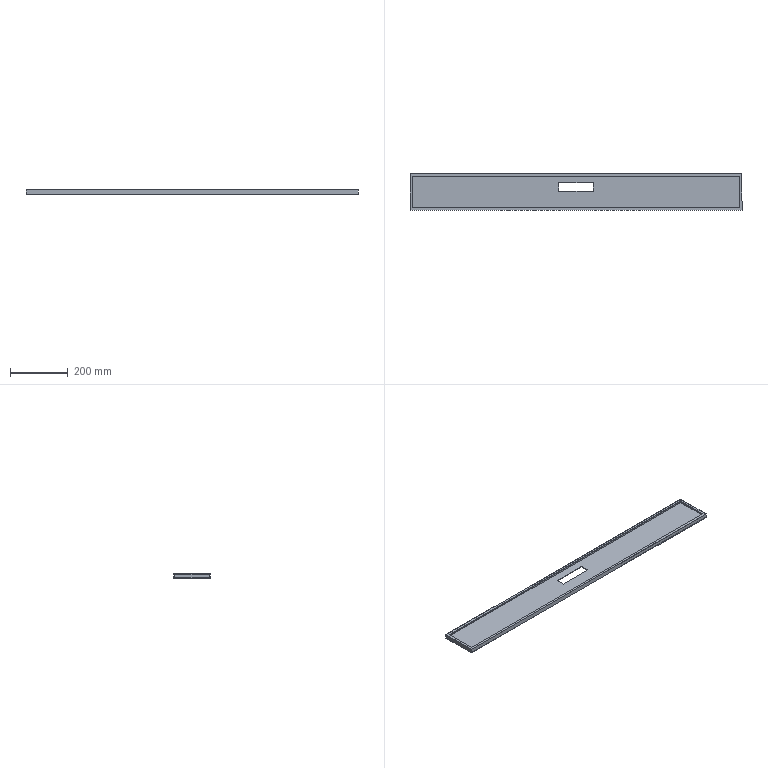Part | SolidWorks | features ICE 2, Extrusion 1, Shell 1 | 1 solid | 20 faces | box 1148 x 125 x 15 mm | volume 375860 mm3 | plane 20
STEP:
#1=CARTESIAN_POINT('',(0.,125.,15.));
#2=VERTEX_POINT('',#1);
#3=CARTESIAN_POINT('',(0.,0.,15.));
#4=VERTEX_POINT('',#3);
#5=CARTESIAN_POINT('',(0.,0.,15.));
#6=DIRECTION('',(0.,-1.,0.));
#7=VECTOR('',#6,1000.);
#8=LINE('',#5,#7);
#9=EDGE_CURVE('',#2,#4,#8,.T.);
#10=ORIENTED_EDGE('',*,*,#9,.T.);
#11=CARTESIAN_POINT('',(1148.,0.,15.));
#12=VERTEX_POINT('',#11);
#13=CARTESIAN_POINT('',(0.,0.,15.));
#14=DIRECTION('',(1.,0.,0.));
#15=VECTOR('',#14,1000.);
#16=LINE('',#13,#15);
#17=EDGE_CURVE('',#4,#12,#16,.T.);
#18=ORIENTED_EDGE('',*,*,#17,.T.);
#19=CARTESIAN_POINT('',(1148.,125.,15.));
#20=VERTEX_POINT('',#19);
#21=CARTESIAN_POINT('',(1148.,0.,15.));
#22=DIRECTION('',(0.,1.,0.));
#23=VECTOR('',#22,1000.);
#24=LINE('',#21,#23);
#25=EDGE_CURVE('',#12,#20,#24,.T.);
#26=ORIENTED_EDGE('',*,*,#25,.T.);
#27=CARTESIAN_POINT('',(0.,125.,15.));
#28=DIRECTION('',(-1.,0.,0.));
#29=VECTOR('',#28,1000.);
#30=LINE('',#27,#29);
#31=EDGE_CURVE('',#20,#2,#30,.T.);
#32=ORIENTED_EDGE('',*,*,#31,.T.);
#33=EDGE_LOOP('',(#10,#18,#26,#32));
#34=FACE_OUTER_BOUND('',#33,.T.);
#35=CARTESIAN_POINT('',(1140.,117.,15.));
#36=VERTEX_POINT('',#35);
#37=CARTESIAN_POINT('',(8.,117.,15.));
#38=VERTEX_POINT('',#37);
#39=CARTESIAN_POINT('',(8.,117.,15.));
#40=DIRECTION('',(-1.,0.,0.));
#41=VECTOR('',#40,1000.);
#42=LINE('',#39,#41);
#43=EDGE_CURVE('',#36,#38,#42,.T.);
#44=ORIENTED_EDGE('',*,*,#43,.F.);
#45=CARTESIAN_POINT('',(1140.,8.,15.));
#46=VERTEX_POINT('',#45);
#47=CARTESIAN_POINT('',(1140.,117.,15.));
#48=DIRECTION('',(0.,1.,0.));
#49=VECTOR('',#48,1000.);
#50=LINE('',#47,#49);
#51=EDGE_CURVE('',#46,#36,#50,.T.);
#52=ORIENTED_EDGE('',*,*,#51,.F.);
#53=CARTESIAN_POINT('',(8.,8.,15.));
#54=VERTEX_POINT('',#53);
#55=CARTESIAN_POINT('',(8.,8.,15.));
#56=DIRECTION('',(1.,0.,0.));
#57=VECTOR('',#56,1000.);
#58=LINE('',#55,#57);
#59=EDGE_CURVE('',#54,#46,#58,.T.);
#60=ORIENTED_EDGE('',*,*,#59,.F.);
#61=CARTESIAN_POINT('',(8.,117.,15.));
#62=DIRECTION('',(0.,-1.,0.));
#63=VECTOR('',#62,1000.);
#64=LINE('',#61,#63);
#65=EDGE_CURVE('',#38,#54,#64,.T.);
#66=ORIENTED_EDGE('',*,*,#65,.F.);
#67=EDGE_LOOP('',(#44,#52,#60,#66));
#68=FACE_BOUND('',#67,.T.);
#69=CARTESIAN_POINT('',(0.,125.,15.));
#70=DIRECTION('',(0.,0.,-1.));
#71=DIRECTION('',(-1.,0.,0.));
#72=AXIS2_PLACEMENT_3D('',#69,#70,#71);
#73=PLANE('',#72);
#74=ADVANCED_FACE('',(#34,#68),#73,.F.);
#75=CARTESIAN_POINT('',(0.,125.,0.));
#76=VERTEX_POINT('',#75);
#77=CARTESIAN_POINT('',(0.,125.,15.));
#78=DIRECTION('',(0.,0.,-1.));
#79=VECTOR('',#78,1000.);
#80=LINE('',#77,#79);
#81=EDGE_CURVE('',#2,#76,#80,.T.);
#82=ORIENTED_EDGE('',*,*,#81,.T.);
#83=CARTESIAN_POINT('',(0.,0.,0.));
#84=VERTEX_POINT('',#83);
#85=CARTESIAN_POINT('',(0.,0.,0.));
#86=DIRECTION('',(0.,-1.,0.));
#87=VECTOR('',#86,1000.);
#88=LINE('',#85,#87);
#89=EDGE_CURVE('',#76,#84,#88,.T.);
#90=ORIENTED_EDGE('',*,*,#89,.T.);
#91=CARTESIAN_POINT('',(0.,0.,15.));
#92=DIRECTION('',(0.,0.,-1.));
#93=VECTOR('',#92,1000.);
#94=LINE('',#91,#93);
#95=EDGE_CURVE('',#4,#84,#94,.T.);
#96=ORIENTED_EDGE('',*,*,#95,.F.);
#97=ORIENTED_EDGE('',*,*,#9,.F.);
#98=EDGE_LOOP('',(#82,#90,#96,#97));
#99=FACE_OUTER_BOUND('',#98,.T.);
#100=CARTESIAN_POINT('',(0.,0.,15.));
#101=DIRECTION('',(1.,0.,0.));
#102=DIRECTION('',(0.,0.,-1.));
#103=AXIS2_PLACEMENT_3D('',#100,#101,#102);
#104=PLANE('',#103);
#105=ADVANCED_FACE('',(#99),#104,.F.);
#106=ORIENTED_EDGE('',*,*,#95,.T.);
#107=CARTESIAN_POINT('',(1148.,0.,0.));
#108=VERTEX_POINT('',#107);
#109=CARTESIAN_POINT('',(0.,0.,0.));
#110=DIRECTION('',(1.,0.,0.));
#111=VECTOR('',#110,1000.);
#112=LINE('',#109,#111);
#113=EDGE_CURVE('',#84,#108,#112,.T.);
#114=ORIENTED_EDGE('',*,*,#113,.T.);
#115=CARTESIAN_POINT('',(1148.,0.,15.));
#116=DIRECTION('',(0.,0.,-1.));
#117=VECTOR('',#116,1000.);
#118=LINE('',#115,#117);
#119=EDGE_CURVE('',#12,#108,#118,.T.);
#120=ORIENTED_EDGE('',*,*,#119,.F.);
#121=ORIENTED_EDGE('',*,*,#17,.F.);
#122=EDGE_LOOP('',(#106,#114,#120,#121));
#123=FACE_OUTER_BOUND('',#122,.T.);
#124=CARTESIAN_POINT('',(0.,0.,15.));
#125=DIRECTION('',(0.,1.,0.));
#126=DIRECTION('',(0.,0.,1.));
#127=AXIS2_PLACEMENT_3D('',#124,#125,#126);
#128=PLANE('',#127);
#129=ADVANCED_FACE('',(#123),#128,.F.);
#130=ORIENTED_EDGE('',*,*,#119,.T.);
#131=CARTESIAN_POINT('',(1148.,125.,0.));
#132=VERTEX_POINT('',#131);
#133=CARTESIAN_POINT('',(1148.,0.,0.));
#134=DIRECTION('',(0.,1.,0.));
#135=VECTOR('',#134,1000.);
#136=LINE('',#133,#135);
#137=EDGE_CURVE('',#108,#132,#136,.T.);
#138=ORIENTED_EDGE('',*,*,#137,.T.);
#139=CARTESIAN_POINT('',(1148.,125.,15.));
#140=DIRECTION('',(0.,0.,-1.));
#141=VECTOR('',#140,1000.);
#142=LINE('',#139,#141);
#143=EDGE_CURVE('',#20,#132,#142,.T.);
#144=ORIENTED_EDGE('',*,*,#143,.F.);
#145=ORIENTED_EDGE('',*,*,#25,.F.);
#146=EDGE_LOOP('',(#130,#138,#144,#145));
#147=FACE_OUTER_BOUND('',#146,.T.);
#148=CARTESIAN_POINT('',(1148.,0.,15.));
#149=DIRECTION('',(-1.,0.,0.));
#150=DIRECTION('',(0.,-1.,0.));
#151=AXIS2_PLACEMENT_3D('',#148,#149,#150);
#152=PLANE('',#151);
#153=ADVANCED_FACE('',(#147),#152,.F.);
#154=ORIENTED_EDGE('',*,*,#143,.T.);
#155=CARTESIAN_POINT('',(0.,125.,0.));
#156=DIRECTION('',(-1.,0.,0.));
#157=VECTOR('',#156,1000.);
#158=LINE('',#155,#157);
#159=EDGE_CURVE('',#132,#76,#158,.T.);
#160=ORIENTED_EDGE('',*,*,#159,.T.);
#161=ORIENTED_EDGE('',*,*,#81,.F.);
#162=ORIENTED_EDGE('',*,*,#31,.F.);
#163=EDGE_LOOP('',(#154,#160,#161,#162));
#164=FACE_OUTER_BOUND('',#163,.T.);
#165=CARTESIAN_POINT('',(0.,125.,15.));
#166=DIRECTION('',(0.,-1.,0.));
#167=DIRECTION('',(0.,0.,-1.));
#168=AXIS2_PLACEMENT_3D('',#165,#166,#167);
#169=PLANE('',#168);
#170=ADVANCED_FACE('',(#164),#169,.F.);
#171=CARTESIAN_POINT('',(634.,95.,0.));
#172=VERTEX_POINT('',#171);
#173=CARTESIAN_POINT('',(634.,65.,0.));
#174=VERTEX_POINT('',#173);
#175=CARTESIAN_POINT('',(634.,95.,0.));
#176=DIRECTION('',(0.,-1.,0.));
#177=VECTOR('',#176,1000.);
#178=LINE('',#175,#177);
#179=EDGE_CURVE('',#172,#174,#178,.T.);
#180=ORIENTED_EDGE('',*,*,#179,.F.);
#181=CARTESIAN_POINT('',(514.,95.,0.));
#182=VERTEX_POINT('',#181);
#183=CARTESIAN_POINT('',(634.,95.,0.));
#184=DIRECTION('',(1.,0.,0.));
#185=VECTOR('',#184,1000.);
#186=LINE('',#183,#185);
#187=EDGE_CURVE('',#182,#172,#186,.T.);
#188=ORIENTED_EDGE('',*,*,#187,.F.);
#189=CARTESIAN_POINT('',(514.,65.,0.));
#190=VERTEX_POINT('',#189);
#191=CARTESIAN_POINT('',(514.,95.,0.));
#192=DIRECTION('',(0.,1.,0.));
#193=VECTOR('',#192,1000.);
#194=LINE('',#191,#193);
#195=EDGE_CURVE('',#190,#182,#194,.T.);
#196=ORIENTED_EDGE('',*,*,#195,.F.);
#197=CARTESIAN_POINT('',(634.,65.,0.));
#198=DIRECTION('',(-1.,0.,0.));
#199=VECTOR('',#198,1000.);
#200=LINE('',#197,#199);
#201=EDGE_CURVE('',#174,#190,#200,.T.);
#202=ORIENTED_EDGE('',*,*,#201,.F.);
#203=EDGE_LOOP('',(#180,#188,#196,#202));
#204=FACE_BOUND('',#203,.T.);
#205=ORIENTED_EDGE('',*,*,#89,.F.);
#206=ORIENTED_EDGE('',*,*,#159,.F.);
#207=ORIENTED_EDGE('',*,*,#137,.F.);
#208=ORIENTED_EDGE('',*,*,#113,.F.);
#209=EDGE_LOOP('',(#205,#206,#207,#208));
#210=FACE_OUTER_BOUND('',#209,.T.);
#211=CARTESIAN_POINT('',(0.,125.,0.));
#212=DIRECTION('',(0.,0.,-1.));
#213=DIRECTION('',(-1.,0.,0.));
#214=AXIS2_PLACEMENT_3D('',#211,#212,#213);
#215=PLANE('',#214);
#216=ADVANCED_FACE('',(#204,#210),#215,.T.);
#217=CARTESIAN_POINT('',(2.,123.,13.));
#218=VERTEX_POINT('',#217);
#219=CARTESIAN_POINT('',(2.,2.,13.));
#220=VERTEX_POINT('',#219);
#221=CARTESIAN_POINT('',(2.,0.,13.));
#222=DIRECTION('',(0.,-1.,0.));
#223=VECTOR('',#222,1000.);
#224=LINE('',#221,#223);
#225=EDGE_CURVE('',#218,#220,#224,.T.);
#226=ORIENTED_EDGE('',*,*,#225,.F.);
#227=CARTESIAN_POINT('',(1146.,123.,13.));
#228=VERTEX_POINT('',#227);
#229=CARTESIAN_POINT('',(0.,123.,13.));
#230=DIRECTION('',(-1.,0.,0.));
#231=VECTOR('',#230,1000.);
#232=LINE('',#229,#231);
#233=EDGE_CURVE('',#228,#218,#232,.T.);
#234=ORIENTED_EDGE('',*,*,#233,.F.);
#235=CARTESIAN_POINT('',(1146.,2.,13.));
#236=VERTEX_POINT('',#235);
#237=CARTESIAN_POINT('',(1146.,0.,13.));
#238=DIRECTION('',(0.,1.,0.));
#239=VECTOR('',#238,1000.);
#240=LINE('',#237,#239);
#241=EDGE_CURVE('',#236,#228,#240,.T.);
#242=ORIENTED_EDGE('',*,*,#241,.F.);
#243=CARTESIAN_POINT('',(0.,2.,13.));
#244=DIRECTION('',(1.,0.,0.));
#245=VECTOR('',#244,1000.);
#246=LINE('',#243,#245);
#247=EDGE_CURVE('',#220,#236,#246,.T.);
#248=ORIENTED_EDGE('',*,*,#247,.F.);
#249=EDGE_LOOP('',(#226,#234,#242,#248));
#250=FACE_OUTER_BOUND('',#249,.T.);
#251=CARTESIAN_POINT('',(1140.,8.,13.));
#252=VERTEX_POINT('',#251);
#253=CARTESIAN_POINT('',(1140.,117.,13.));
#254=VERTEX_POINT('',#253);
#255=CARTESIAN_POINT('',(1140.,117.,13.));
#256=DIRECTION('',(0.,1.,0.));
#257=VECTOR('',#256,1000.);
#258=LINE('',#255,#257);
#259=EDGE_CURVE('',#252,#254,#258,.T.);
#260=ORIENTED_EDGE('',*,*,#259,.T.);
#261=CARTESIAN_POINT('',(8.,117.,13.));
#262=VERTEX_POINT('',#261);
#263=CARTESIAN_POINT('',(8.,117.,13.));
#264=DIRECTION('',(-1.,0.,0.));
#265=VECTOR('',#264,1000.);
#266=LINE('',#263,#265);
#267=EDGE_CURVE('',#254,#262,#266,.T.);
#268=ORIENTED_EDGE('',*,*,#267,.T.);
#269=CARTESIAN_POINT('',(8.,8.,13.));
#270=VERTEX_POINT('',#269);
#271=CARTESIAN_POINT('',(8.,117.,13.));
#272=DIRECTION('',(0.,-1.,0.));
#273=VECTOR('',#272,1000.);
#274=LINE('',#271,#273);
#275=EDGE_CURVE('',#262,#270,#274,.T.);
#276=ORIENTED_EDGE('',*,*,#275,.T.);
#277=CARTESIAN_POINT('',(8.,8.,13.));
#278=DIRECTION('',(1.,0.,0.));
#279=VECTOR('',#278,1000.);
#280=LINE('',#277,#279);
#281=EDGE_CURVE('',#270,#252,#280,.T.);
#282=ORIENTED_EDGE('',*,*,#281,.T.);
#283=EDGE_LOOP('',(#260,#268,#276,#282));
#284=FACE_BOUND('',#283,.T.);
#285=CARTESIAN_POINT('',(0.,0.,13.));
#286=DIRECTION('',(0.,0.,1.));
#287=DIRECTION('',(1.,0.,0.));
#288=AXIS2_PLACEMENT_3D('',#285,#286,#287);
#289=PLANE('',#288);
#290=ADVANCED_FACE('',(#250,#284),#289,.F.);
#291=ORIENTED_EDGE('',*,*,#43,.T.);
#292=CARTESIAN_POINT('',(8.,117.,13.));
#293=DIRECTION('',(0.,0.,1.));
#294=VECTOR('',#293,1000.);
#295=LINE('',#292,#294);
#296=EDGE_CURVE('',#262,#38,#295,.T.);
#297=ORIENTED_EDGE('',*,*,#296,.F.);
#298=ORIENTED_EDGE('',*,*,#267,.F.);
#299=CARTESIAN_POINT('',(1140.,117.,13.));
#300=DIRECTION('',(0.,0.,1.));
#301=VECTOR('',#300,1000.);
#302=LINE('',#299,#301);
#303=EDGE_CURVE('',#254,#36,#302,.T.);
#304=ORIENTED_EDGE('',*,*,#303,.T.);
#305=EDGE_LOOP('',(#291,#297,#298,#304));
#306=FACE_OUTER_BOUND('',#305,.T.);
#307=CARTESIAN_POINT('',(8.,117.,13.));
#308=DIRECTION('',(0.,1.,0.));
#309=DIRECTION('',(0.,0.,1.));
#310=AXIS2_PLACEMENT_3D('',#307,#308,#309);
#311=PLANE('',#310);
#312=ADVANCED_FACE('',(#306),#311,.F.);
#313=ORIENTED_EDGE('',*,*,#51,.T.);
#314=ORIENTED_EDGE('',*,*,#303,.F.);
#315=ORIENTED_EDGE('',*,*,#259,.F.);
#316=CARTESIAN_POINT('',(1140.,8.,13.));
#317=DIRECTION('',(0.,0.,1.));
#318=VECTOR('',#317,1000.);
#319=LINE('',#316,#318);
#320=EDGE_CURVE('',#252,#46,#319,.T.);
#321=ORIENTED_EDGE('',*,*,#320,.T.);
#322=EDGE_LOOP('',(#313,#314,#315,#321));
#323=FACE_OUTER_BOUND('',#322,.T.);
#324=CARTESIAN_POINT('',(1140.,117.,13.));
#325=DIRECTION('',(1.,0.,0.));
#326=DIRECTION('',(0.,0.,-1.));
#327=AXIS2_PLACEMENT_3D('',#324,#325,#326);
#328=PLANE('',#327);
#329=ADVANCED_FACE('',(#323),#328,.F.);
#330=ORIENTED_EDGE('',*,*,#59,.T.);
#331=ORIENTED_EDGE('',*,*,#320,.F.);
#332=ORIENTED_EDGE('',*,*,#281,.F.);
#333=CARTESIAN_POINT('',(8.,8.,13.));
#334=DIRECTION('',(0.,0.,1.));
#335=VECTOR('',#334,1000.);
#336=LINE('',#333,#335);
#337=EDGE_CURVE('',#270,#54,#336,.T.);
#338=ORIENTED_EDGE('',*,*,#337,.T.);
#339=EDGE_LOOP('',(#330,#331,#332,#338));
#340=FACE_OUTER_BOUND('',#339,.T.);
#341=CARTESIAN_POINT('',(8.,8.,13.));
#342=DIRECTION('',(0.,-1.,0.));
#343=DIRECTION('',(1.,0.,0.));
#344=AXIS2_PLACEMENT_3D('',#341,#342,#343);
#345=PLANE('',#344);
#346=ADVANCED_FACE('',(#340),#345,.F.);
#347=ORIENTED_EDGE('',*,*,#65,.T.);
#348=ORIENTED_EDGE('',*,*,#337,.F.);
#349=ORIENTED_EDGE('',*,*,#275,.F.);
#350=ORIENTED_EDGE('',*,*,#296,.T.);
#351=EDGE_LOOP('',(#347,#348,#349,#350));
#352=FACE_OUTER_BOUND('',#351,.T.);
#353=CARTESIAN_POINT('',(8.,117.,13.));
#354=DIRECTION('',(-1.,0.,0.));
#355=DIRECTION('',(0.,-1.,0.));
#356=AXIS2_PLACEMENT_3D('',#353,#354,#355);
#357=PLANE('',#356);
#358=ADVANCED_FACE('',(#352),#357,.F.);
#359=CARTESIAN_POINT('',(514.,95.,2.));
#360=VERTEX_POINT('',#359);
#361=CARTESIAN_POINT('',(634.,95.,2.));
#362=VERTEX_POINT('',#361);
#363=CARTESIAN_POINT('',(0.,95.,2.));
#364=DIRECTION('',(1.,0.,0.));
#365=VECTOR('',#364,1000.);
#366=LINE('',#363,#365);
#367=EDGE_CURVE('',#360,#362,#366,.T.);
#368=ORIENTED_EDGE('',*,*,#367,.T.);
#369=CARTESIAN_POINT('',(634.,65.,2.));
#370=VERTEX_POINT('',#369);
#371=CARTESIAN_POINT('',(634.,125.,2.));
#372=DIRECTION('',(0.,-1.,0.));
#373=VECTOR('',#372,1000.);
#374=LINE('',#371,#373);
#375=EDGE_CURVE('',#362,#370,#374,.T.);
#376=ORIENTED_EDGE('',*,*,#375,.T.);
#377=CARTESIAN_POINT('',(514.,65.,2.));
#378=VERTEX_POINT('',#377);
#379=CARTESIAN_POINT('',(0.,65.,2.));
#380=DIRECTION('',(-1.,0.,0.));
#381=VECTOR('',#380,1000.);
#382=LINE('',#379,#381);
#383=EDGE_CURVE('',#370,#378,#382,.T.);
#384=ORIENTED_EDGE('',*,*,#383,.T.);
#385=CARTESIAN_POINT('',(514.,125.,2.));
#386=DIRECTION('',(0.,1.,0.));
#387=VECTOR('',#386,1000.);
#388=LINE('',#385,#387);
#389=EDGE_CURVE('',#378,#360,#388,.T.);
#390=ORIENTED_EDGE('',*,*,#389,.T.);
#391=EDGE_LOOP('',(#368,#376,#384,#390));
#392=FACE_BOUND('',#391,.T.);
#393=CARTESIAN_POINT('',(2.,123.,2.));
#394=VERTEX_POINT('',#393);
#395=CARTESIAN_POINT('',(2.,2.,2.));
#396=VERTEX_POINT('',#395);
#397=CARTESIAN_POINT('',(2.,125.,2.));
#398=DIRECTION('',(0.,-1.,0.));
#399=VECTOR('',#398,1000.);
#400=LINE('',#397,#399);
#401=EDGE_CURVE('',#394,#396,#400,.T.);
#402=ORIENTED_EDGE('',*,*,#401,.T.);
#403=CARTESIAN_POINT('',(1146.,2.,2.));
#404=VERTEX_POINT('',#403);
#405=CARTESIAN_POINT('',(0.,2.,2.));
#406=DIRECTION('',(1.,0.,0.));
#407=VECTOR('',#406,1000.);
#408=LINE('',#405,#407);
#409=EDGE_CURVE('',#396,#404,#408,.T.);
#410=ORIENTED_EDGE('',*,*,#409,.T.);
#411=CARTESIAN_POINT('',(1146.,123.,2.));
#412=VERTEX_POINT('',#411);
#413=CARTESIAN_POINT('',(1146.,125.,2.));
#414=DIRECTION('',(0.,1.,0.));
#415=VECTOR('',#414,1000.);
#416=LINE('',#413,#415);
#417=EDGE_CURVE('',#404,#412,#416,.T.);
#418=ORIENTED_EDGE('',*,*,#417,.T.);
#419=CARTESIAN_POINT('',(0.,123.,2.));
#420=DIRECTION('',(-1.,0.,0.));
#421=VECTOR('',#420,1000.);
#422=LINE('',#419,#421);
#423=EDGE_CURVE('',#412,#394,#422,.T.);
#424=ORIENTED_EDGE('',*,*,#423,.T.);
#425=EDGE_LOOP('',(#402,#410,#418,#424));
#426=FACE_OUTER_BOUND('',#425,.T.);
#427=CARTESIAN_POINT('',(0.,125.,2.));
#428=DIRECTION('',(0.,0.,-1.));
#429=DIRECTION('',(-1.,0.,0.));
#430=AXIS2_PLACEMENT_3D('',#427,#428,#429);
#431=PLANE('',#430);
#432=ADVANCED_FACE('',(#392,#426),#431,.F.);
#433=CARTESIAN_POINT('',(1146.,123.,15.));
#434=DIRECTION('',(0.,0.,-1.));
#435=VECTOR('',#434,1000.);
#436=LINE('',#433,#435);
#437=EDGE_CURVE('',#228,#412,#436,.T.);
#438=ORIENTED_EDGE('',*,*,#437,.F.);
#439=ORIENTED_EDGE('',*,*,#233,.T.);
#440=CARTESIAN_POINT('',(2.,123.,15.));
#441=DIRECTION('',(0.,0.,-1.));
#442=VECTOR('',#441,1000.);
#443=LINE('',#440,#442);
#444=EDGE_CURVE('',#218,#394,#443,.T.);
#445=ORIENTED_EDGE('',*,*,#444,.T.);
#446=ORIENTED_EDGE('',*,*,#423,.F.);
#447=EDGE_LOOP('',(#438,#439,#445,#446));
#448=FACE_OUTER_BOUND('',#447,.T.);
#449=CARTESIAN_POINT('',(0.,123.,15.));
#450=DIRECTION('',(0.,-1.,0.));
#451=DIRECTION('',(0.,0.,-1.));
#452=AXIS2_PLACEMENT_3D('',#449,#450,#451);
#453=PLANE('',#452);
#454=ADVANCED_FACE('',(#448),#453,.T.);
#455=CARTESIAN_POINT('',(1146.,2.,15.));
#456=DIRECTION('',(0.,0.,-1.));
#457=VECTOR('',#456,1000.);
#458=LINE('',#455,#457);
#459=EDGE_CURVE('',#236,#404,#458,.T.);
#460=ORIENTED_EDGE('',*,*,#459,.F.);
#461=ORIENTED_EDGE('',*,*,#241,.T.);
#462=ORIENTED_EDGE('',*,*,#437,.T.);
#463=ORIENTED_EDGE('',*,*,#417,.F.);
#464=EDGE_LOOP('',(#460,#461,#462,#463));
#465=FACE_OUTER_BOUND('',#464,.T.);
#466=CARTESIAN_POINT('',(1146.,0.,15.));
#467=DIRECTION('',(-1.,0.,0.));
#468=DIRECTION('',(0.,-1.,0.));
#469=AXIS2_PLACEMENT_3D('',#466,#467,#468);
#470=PLANE('',#469);
#471=ADVANCED_FACE('',(#465),#470,.T.);
#472=CARTESIAN_POINT('',(2.,2.,15.));
#473=DIRECTION('',(0.,0.,-1.));
#474=VECTOR('',#473,1000.);
#475=LINE('',#472,#474);
#476=EDGE_CURVE('',#220,#396,#475,.T.);
#477=ORIENTED_EDGE('',*,*,#476,.F.);
#478=ORIENTED_EDGE('',*,*,#247,.T.);
#479=ORIENTED_EDGE('',*,*,#459,.T.);
#480=ORIENTED_EDGE('',*,*,#409,.F.);
#481=EDGE_LOOP('',(#477,#478,#479,#480));
#482=FACE_OUTER_BOUND('',#481,.T.);
#483=CARTESIAN_POINT('',(0.,2.,15.));
#484=DIRECTION('',(0.,1.,0.));
#485=DIRECTION('',(0.,0.,1.));
#486=AXIS2_PLACEMENT_3D('',#483,#484,#485);
#487=PLANE('',#486);
#488=ADVANCED_FACE('',(#482),#487,.T.);
#489=ORIENTED_EDGE('',*,*,#444,.F.);
#490=ORIENTED_EDGE('',*,*,#225,.T.);
#491=ORIENTED_EDGE('',*,*,#476,.T.);
#492=ORIENTED_EDGE('',*,*,#401,.F.);
#493=EDGE_LOOP('',(#489,#490,#491,#492));
#494=FACE_OUTER_BOUND('',#493,.T.);
#495=CARTESIAN_POINT('',(2.,0.,15.));
#496=DIRECTION('',(1.,0.,0.));
#497=DIRECTION('',(0.,0.,-1.));
#498=AXIS2_PLACEMENT_3D('',#495,#496,#497);
#499=PLANE('',#498);
#500=ADVANCED_FACE('',(#494),#499,.T.);
#501=CARTESIAN_POINT('',(634.,95.,10.));
#502=DIRECTION('',(0.,0.,-1.));
#503=VECTOR('',#502,1000.);
#504=LINE('',#501,#503);
#505=EDGE_CURVE('',#362,#172,#504,.T.);
#506=ORIENTED_EDGE('',*,*,#505,.T.);
#507=ORIENTED_EDGE('',*,*,#179,.T.);
#508=CARTESIAN_POINT('',(634.,65.,10.));
#509=DIRECTION('',(0.,0.,-1.));
#510=VECTOR('',#509,1000.);
#511=LINE('',#508,#510);
#512=EDGE_CURVE('',#370,#174,#511,.T.);
#513=ORIENTED_EDGE('',*,*,#512,.F.);
#514=ORIENTED_EDGE('',*,*,#375,.F.);
#515=EDGE_LOOP('',(#506,#507,#513,#514));
#516=FACE_OUTER_BOUND('',#515,.T.);
#517=CARTESIAN_POINT('',(634.,95.,10.));
#518=DIRECTION('',(1.,0.,0.));
#519=DIRECTION('',(0.,0.,-1.));
#520=AXIS2_PLACEMENT_3D('',#517,#518,#519);
#521=PLANE('',#520);
#522=ADVANCED_FACE('',(#516),#521,.F.);
#523=CARTESIAN_POINT('',(514.,95.,10.));
#524=DIRECTION('',(0.,0.,-1.));
#525=VECTOR('',#524,1000.);
#526=LINE('',#523,#525);
#527=EDGE_CURVE('',#360,#182,#526,.T.);
#528=ORIENTED_EDGE('',*,*,#527,.T.);
#529=ORIENTED_EDGE('',*,*,#187,.T.);
#530=ORIENTED_EDGE('',*,*,#505,.F.);
#531=ORIENTED_EDGE('',*,*,#367,.F.);
#532=EDGE_LOOP('',(#528,#529,#530,#531));
#533=FACE_OUTER_BOUND('',#532,.T.);
#534=CARTESIAN_POINT('',(634.,95.,10.));
#535=DIRECTION('',(0.,1.,0.));
#536=DIRECTION('',(0.,0.,1.));
#537=AXIS2_PLACEMENT_3D('',#534,#535,#536);
#538=PLANE('',#537);
#539=ADVANCED_FACE('',(#533),#538,.F.);
#540=CARTESIAN_POINT('',(514.,65.,10.));
#541=DIRECTION('',(0.,0.,-1.));
#542=VECTOR('',#541,1000.);
#543=LINE('',#540,#542);
#544=EDGE_CURVE('',#378,#190,#543,.T.);
#545=ORIENTED_EDGE('',*,*,#544,.T.);
#546=ORIENTED_EDGE('',*,*,#195,.T.);
#547=ORIENTED_EDGE('',*,*,#527,.F.);
#548=ORIENTED_EDGE('',*,*,#389,.F.);
#549=EDGE_LOOP('',(#545,#546,#547,#548));
#550=FACE_OUTER_BOUND('',#549,.T.);
#551=CARTESIAN_POINT('',(514.,95.,10.));
#552=DIRECTION('',(-1.,0.,0.));
#553=DIRECTION('',(0.,0.,1.));
#554=AXIS2_PLACEMENT_3D('',#551,#552,#553);
#555=PLANE('',#554);
#556=ADVANCED_FACE('',(#550),#555,.F.);
#557=ORIENTED_EDGE('',*,*,#512,.T.);
#558=ORIENTED_EDGE('',*,*,#201,.T.);
#559=ORIENTED_EDGE('',*,*,#544,.F.);
#560=ORIENTED_EDGE('',*,*,#383,.F.);
#561=EDGE_LOOP('',(#557,#558,#559,#560));
#562=FACE_OUTER_BOUND('',#561,.T.);
#563=CARTESIAN_POINT('',(634.,65.,10.));
#564=DIRECTION('',(0.,-1.,0.));
#565=DIRECTION('',(0.,0.,-1.));
#566=AXIS2_PLACEMENT_3D('',#563,#564,#565);
#567=PLANE('',#566);
#568=ADVANCED_FACE('',(#562),#567,.F.);
#569=CLOSED_SHELL('',(#74,#105,#129,#153,#170,#216,#290,#312,#329,#346,#358,#432,#454,#471,#488,#500,#522,#539,#556,#568));
#570=MANIFOLD_SOLID_BREP('',#569);
#571=CARTESIAN_POINT('',(0.,0.,0.));
#572=DIRECTION('',(0.,0.,1.));
#573=DIRECTION('',(1.,0.,0.));
#574=AXIS2_PLACEMENT_3D('',#571,#572,#573);
#575=(LENGTH_UNIT()NAMED_UNIT(*)SI_UNIT(.MILLI.,.METRE.));
#576=UNCERTAINTY_MEASURE_WITH_UNIT(LENGTH_MEASURE(0.00001),#575,'','');
#577=(NAMED_UNIT(*)PLANE_ANGLE_UNIT()SI_UNIT($,.RADIAN.));
#578=(NAMED_UNIT(*)SI_UNIT($,.STERADIAN.)SOLID_ANGLE_UNIT());
#579=(GEOMETRIC_REPRESENTATION_CONTEXT(3)GLOBAL_UNCERTAINTY_ASSIGNED_CONTEXT((#576))GLOBAL_UNIT_ASSIGNED_CONTEXT((#575,#577,#578))REPRESENTATION_CONTEXT('',''));
#580=ADVANCED_BREP_SHAPE_REPRESENTATION('',(#570,#574),#579);